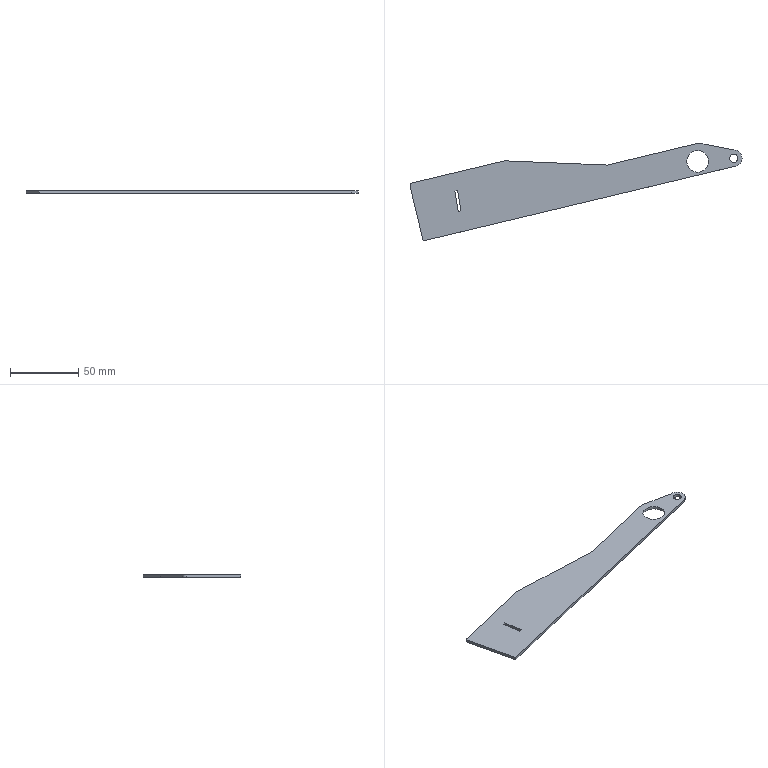Part | STEP file | 1 solid | 19 faces | box 242.784 x 71.457 x 2 mm | volume 14415 mm3 | plane 12 | cylinder 7 | commonest cylinder face diameters 6 x2 12 x2 16 x2 4 x1